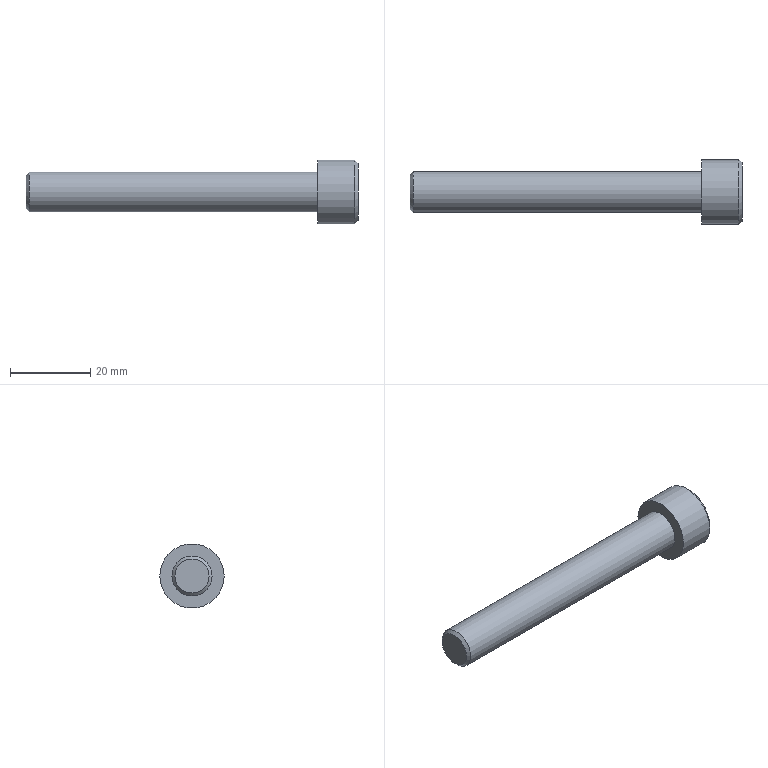Part | STEP file | solid 204 | 1 solid | 14 faces | box 82.5 x 16 x 16 mm | volume 7406 mm3 | plane 10 | cone 2 | cylinder 2 | commonest cylinder face diameters 10 x1 16 x1